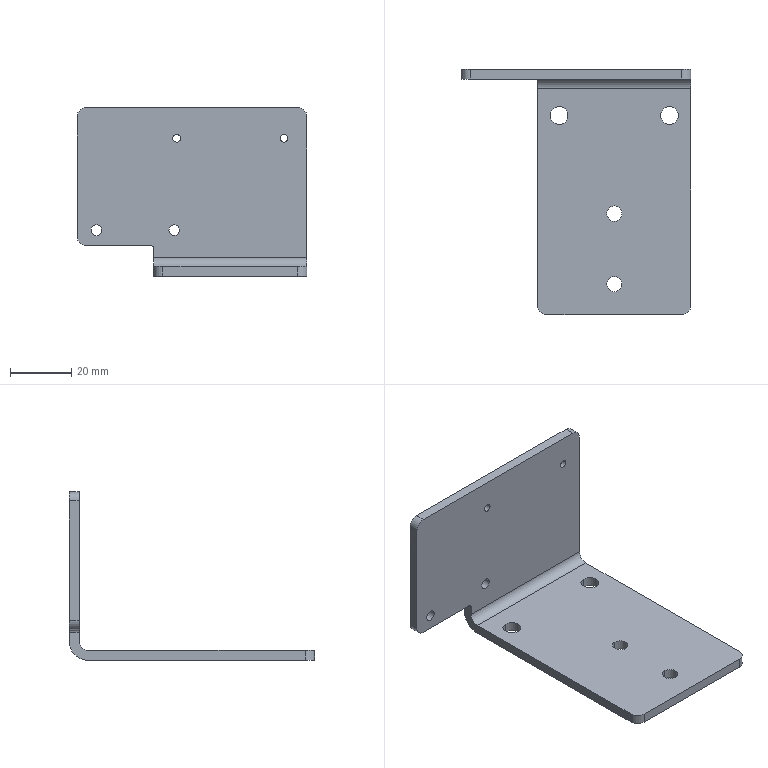Part | STEP file | J014-EBZ05-01-06-Part-1 | 1 solid | 34 faces | box 75 x 80 x 55 mm | volume 23980 mm3 | cylinder 24 | plane 10 | commonest cylinder face diameters 6 x6 2.5 x4 3.5 x4 5 x4 5.8 x4 2 x1
STEP:
#1=CARTESIAN_POINT('',(8.45,0.,15.));
#2=VERTEX_POINT('',#1);
#3=CARTESIAN_POINT('',(4.95,0.,15.));
#4=VERTEX_POINT('',#3);
#5=CARTESIAN_POINT('',(6.7,0.,15.));
#6=DIRECTION('',(0.,-1.,0.));
#7=DIRECTION('',(-1.,0.,0.));
#8=AXIS2_PLACEMENT_3D('',#5,#6,#7);
#9=CIRCLE('',#8,1.75);
#10=EDGE_CURVE('',#2,#4,#9,.T.);
#11=ORIENTED_EDGE('',*,*,#10,.F.);
#12=CARTESIAN_POINT('',(8.45,-3.2,15.));
#13=VERTEX_POINT('',#12);
#14=CARTESIAN_POINT('',(8.45,0.,15.));
#15=DIRECTION('',(0.,-1.,0.));
#16=VECTOR('',#15,1000.);
#17=LINE('',#14,#16);
#18=EDGE_CURVE('',#2,#13,#17,.T.);
#19=ORIENTED_EDGE('',*,*,#18,.T.);
#20=CARTESIAN_POINT('',(4.95,-3.2,15.));
#21=VERTEX_POINT('',#20);
#22=CARTESIAN_POINT('',(6.7,-3.2,15.));
#23=DIRECTION('',(0.,1.,0.));
#24=DIRECTION('',(1.,0.,0.));
#25=AXIS2_PLACEMENT_3D('',#22,#23,#24);
#26=CIRCLE('',#25,1.75);
#27=EDGE_CURVE('',#21,#13,#26,.T.);
#28=ORIENTED_EDGE('',*,*,#27,.F.);
#29=CARTESIAN_POINT('',(4.95,0.,15.));
#30=DIRECTION('',(0.,-1.,0.));
#31=VECTOR('',#30,1000.);
#32=LINE('',#29,#31);
#33=EDGE_CURVE('',#4,#21,#32,.T.);
#34=ORIENTED_EDGE('',*,*,#33,.F.);
#35=EDGE_LOOP('',(#11,#19,#28,#34));
#36=FACE_OUTER_BOUND('',#35,.T.);
#37=CARTESIAN_POINT('',(6.7,0.,15.));
#38=DIRECTION('',(0.,-1.,0.));
#39=DIRECTION('',(-1.,0.,0.));
#40=AXIS2_PLACEMENT_3D('',#37,#38,#39);
#41=CYLINDRICAL_SURFACE('',#40,1.75);
#42=ADVANCED_FACE('',(#36),#41,.F.);
#43=CARTESIAN_POINT('',(-16.95,0.,15.));
#44=VERTEX_POINT('',#43);
#45=CARTESIAN_POINT('',(-20.45,0.,15.));
#46=VERTEX_POINT('',#45);
#47=CARTESIAN_POINT('',(-18.7,0.,15.));
#48=DIRECTION('',(0.,-1.,0.));
#49=DIRECTION('',(-1.,0.,0.));
#50=AXIS2_PLACEMENT_3D('',#47,#48,#49);
#51=CIRCLE('',#50,1.75);
#52=EDGE_CURVE('',#44,#46,#51,.T.);
#53=ORIENTED_EDGE('',*,*,#52,.F.);
#54=CARTESIAN_POINT('',(-16.95,-3.2,15.));
#55=VERTEX_POINT('',#54);
#56=CARTESIAN_POINT('',(-16.95,0.,15.));
#57=DIRECTION('',(0.,-1.,0.));
#58=VECTOR('',#57,1000.);
#59=LINE('',#56,#58);
#60=EDGE_CURVE('',#44,#55,#59,.T.);
#61=ORIENTED_EDGE('',*,*,#60,.T.);
#62=CARTESIAN_POINT('',(-20.45,-3.2,15.));
#63=VERTEX_POINT('',#62);
#64=CARTESIAN_POINT('',(-18.7,-3.2,15.));
#65=DIRECTION('',(0.,1.,0.));
#66=DIRECTION('',(1.,0.,0.));
#67=AXIS2_PLACEMENT_3D('',#64,#65,#66);
#68=CIRCLE('',#67,1.75);
#69=EDGE_CURVE('',#63,#55,#68,.T.);
#70=ORIENTED_EDGE('',*,*,#69,.F.);
#71=CARTESIAN_POINT('',(-20.45,0.,15.));
#72=DIRECTION('',(0.,-1.,0.));
#73=VECTOR('',#72,1000.);
#74=LINE('',#71,#73);
#75=EDGE_CURVE('',#46,#63,#74,.T.);
#76=ORIENTED_EDGE('',*,*,#75,.F.);
#77=EDGE_LOOP('',(#53,#61,#70,#76));
#78=FACE_OUTER_BOUND('',#77,.T.);
#79=CARTESIAN_POINT('',(-18.7,0.,15.));
#80=DIRECTION('',(0.,-1.,0.));
#81=DIRECTION('',(-1.,0.,0.));
#82=AXIS2_PLACEMENT_3D('',#79,#80,#81);
#83=CYLINDRICAL_SURFACE('',#82,1.75);
#84=ADVANCED_FACE('',(#78),#83,.F.);
#85=CARTESIAN_POINT('',(43.75,0.,45.));
#86=VERTEX_POINT('',#85);
#87=CARTESIAN_POINT('',(41.25,0.,45.));
#88=VERTEX_POINT('',#87);
#89=CARTESIAN_POINT('',(42.5,0.,45.));
#90=DIRECTION('',(0.,-1.,0.));
#91=DIRECTION('',(-1.,0.,0.));
#92=AXIS2_PLACEMENT_3D('',#89,#90,#91);
#93=CIRCLE('',#92,1.25);
#94=EDGE_CURVE('',#86,#88,#93,.T.);
#95=ORIENTED_EDGE('',*,*,#94,.F.);
#96=CARTESIAN_POINT('',(43.75,-3.2,45.));
#97=VERTEX_POINT('',#96);
#98=CARTESIAN_POINT('',(43.75,0.,45.));
#99=DIRECTION('',(0.,-1.,0.));
#100=VECTOR('',#99,1000.);
#101=LINE('',#98,#100);
#102=EDGE_CURVE('',#86,#97,#101,.T.);
#103=ORIENTED_EDGE('',*,*,#102,.T.);
#104=CARTESIAN_POINT('',(41.25,-3.2,45.));
#105=VERTEX_POINT('',#104);
#106=CARTESIAN_POINT('',(42.5,-3.2,45.));
#107=DIRECTION('',(0.,1.,0.));
#108=DIRECTION('',(1.,0.,0.));
#109=AXIS2_PLACEMENT_3D('',#106,#107,#108);
#110=CIRCLE('',#109,1.25);
#111=EDGE_CURVE('',#105,#97,#110,.T.);
#112=ORIENTED_EDGE('',*,*,#111,.F.);
#113=CARTESIAN_POINT('',(41.25,0.,45.));
#114=DIRECTION('',(0.,-1.,0.));
#115=VECTOR('',#114,1000.);
#116=LINE('',#113,#115);
#117=EDGE_CURVE('',#88,#105,#116,.T.);
#118=ORIENTED_EDGE('',*,*,#117,.F.);
#119=EDGE_LOOP('',(#95,#103,#112,#118));
#120=FACE_OUTER_BOUND('',#119,.T.);
#121=CARTESIAN_POINT('',(42.5,0.,45.));
#122=DIRECTION('',(0.,-1.,0.));
#123=DIRECTION('',(-1.,0.,0.));
#124=AXIS2_PLACEMENT_3D('',#121,#122,#123);
#125=CYLINDRICAL_SURFACE('',#124,1.25);
#126=ADVANCED_FACE('',(#120),#125,.F.);
#127=CARTESIAN_POINT('',(8.75,0.,45.));
#128=VERTEX_POINT('',#127);
#129=CARTESIAN_POINT('',(6.25,0.,45.));
#130=VERTEX_POINT('',#129);
#131=CARTESIAN_POINT('',(7.5,0.,45.));
#132=DIRECTION('',(0.,-1.,0.));
#133=DIRECTION('',(-1.,0.,0.));
#134=AXIS2_PLACEMENT_3D('',#131,#132,#133);
#135=CIRCLE('',#134,1.25);
#136=EDGE_CURVE('',#128,#130,#135,.T.);
#137=ORIENTED_EDGE('',*,*,#136,.F.);
#138=CARTESIAN_POINT('',(8.75,-3.2,45.));
#139=VERTEX_POINT('',#138);
#140=CARTESIAN_POINT('',(8.75,0.,45.));
#141=DIRECTION('',(0.,-1.,0.));
#142=VECTOR('',#141,1000.);
#143=LINE('',#140,#142);
#144=EDGE_CURVE('',#128,#139,#143,.T.);
#145=ORIENTED_EDGE('',*,*,#144,.T.);
#146=CARTESIAN_POINT('',(6.25,-3.2,45.));
#147=VERTEX_POINT('',#146);
#148=CARTESIAN_POINT('',(7.5,-3.2,45.));
#149=DIRECTION('',(0.,1.,0.));
#150=DIRECTION('',(1.,0.,0.));
#151=AXIS2_PLACEMENT_3D('',#148,#149,#150);
#152=CIRCLE('',#151,1.25);
#153=EDGE_CURVE('',#147,#139,#152,.T.);
#154=ORIENTED_EDGE('',*,*,#153,.F.);
#155=CARTESIAN_POINT('',(6.25,0.,45.));
#156=DIRECTION('',(0.,-1.,0.));
#157=VECTOR('',#156,1000.);
#158=LINE('',#155,#157);
#159=EDGE_CURVE('',#130,#147,#158,.T.);
#160=ORIENTED_EDGE('',*,*,#159,.F.);
#161=EDGE_LOOP('',(#137,#145,#154,#160));
#162=FACE_OUTER_BOUND('',#161,.T.);
#163=CARTESIAN_POINT('',(7.5,0.,45.));
#164=DIRECTION('',(0.,-1.,0.));
#165=DIRECTION('',(-1.,0.,0.));
#166=AXIS2_PLACEMENT_3D('',#163,#164,#165);
#167=CYLINDRICAL_SURFACE('',#166,1.25);
#168=ADVANCED_FACE('',(#162),#167,.F.);
#169=CARTESIAN_POINT('',(25.,-67.5,3.2));
#170=VERTEX_POINT('',#169);
#171=CARTESIAN_POINT('',(25.,-72.5,3.2));
#172=VERTEX_POINT('',#171);
#173=CARTESIAN_POINT('',(25.,-70.,3.2));
#174=DIRECTION('',(0.,0.,-1.));
#175=DIRECTION('',(0.,-1.,0.));
#176=AXIS2_PLACEMENT_3D('',#173,#174,#175);
#177=CIRCLE('',#176,2.5);
#178=EDGE_CURVE('',#170,#172,#177,.T.);
#179=ORIENTED_EDGE('',*,*,#178,.F.);
#180=CARTESIAN_POINT('',(25.,-67.5,0.));
#181=VERTEX_POINT('',#180);
#182=CARTESIAN_POINT('',(25.,-67.5,3.2));
#183=DIRECTION('',(0.,0.,-1.));
#184=VECTOR('',#183,1000.);
#185=LINE('',#182,#184);
#186=EDGE_CURVE('',#170,#181,#185,.T.);
#187=ORIENTED_EDGE('',*,*,#186,.T.);
#188=CARTESIAN_POINT('',(25.,-72.5,0.));
#189=VERTEX_POINT('',#188);
#190=CARTESIAN_POINT('',(25.,-70.,0.));
#191=DIRECTION('',(0.,0.,1.));
#192=DIRECTION('',(0.,1.,0.));
#193=AXIS2_PLACEMENT_3D('',#190,#191,#192);
#194=CIRCLE('',#193,2.5);
#195=EDGE_CURVE('',#189,#181,#194,.T.);
#196=ORIENTED_EDGE('',*,*,#195,.F.);
#197=CARTESIAN_POINT('',(25.,-72.5,3.2));
#198=DIRECTION('',(0.,0.,-1.));
#199=VECTOR('',#198,1000.);
#200=LINE('',#197,#199);
#201=EDGE_CURVE('',#172,#189,#200,.T.);
#202=ORIENTED_EDGE('',*,*,#201,.F.);
#203=EDGE_LOOP('',(#179,#187,#196,#202));
#204=FACE_OUTER_BOUND('',#203,.T.);
#205=CARTESIAN_POINT('',(25.,-70.,3.2));
#206=DIRECTION('',(0.,0.,-1.));
#207=DIRECTION('',(0.,-1.,0.));
#208=AXIS2_PLACEMENT_3D('',#205,#206,#207);
#209=CYLINDRICAL_SURFACE('',#208,2.5);
#210=ADVANCED_FACE('',(#204),#209,.F.);
#211=CARTESIAN_POINT('',(25.,-44.5,3.2));
#212=VERTEX_POINT('',#211);
#213=CARTESIAN_POINT('',(25.,-49.5,3.2));
#214=VERTEX_POINT('',#213);
#215=CARTESIAN_POINT('',(25.,-47.,3.2));
#216=DIRECTION('',(0.,0.,-1.));
#217=DIRECTION('',(0.,-1.,0.));
#218=AXIS2_PLACEMENT_3D('',#215,#216,#217);
#219=CIRCLE('',#218,2.5);
#220=EDGE_CURVE('',#212,#214,#219,.T.);
#221=ORIENTED_EDGE('',*,*,#220,.F.);
#222=CARTESIAN_POINT('',(25.,-44.5,0.));
#223=VERTEX_POINT('',#222);
#224=CARTESIAN_POINT('',(25.,-44.5,3.2));
#225=DIRECTION('',(0.,0.,-1.));
#226=VECTOR('',#225,1000.);
#227=LINE('',#224,#226);
#228=EDGE_CURVE('',#212,#223,#227,.T.);
#229=ORIENTED_EDGE('',*,*,#228,.T.);
#230=CARTESIAN_POINT('',(25.,-49.5,0.));
#231=VERTEX_POINT('',#230);
#232=CARTESIAN_POINT('',(25.,-47.,0.));
#233=DIRECTION('',(0.,0.,1.));
#234=DIRECTION('',(0.,1.,0.));
#235=AXIS2_PLACEMENT_3D('',#232,#233,#234);
#236=CIRCLE('',#235,2.5);
#237=EDGE_CURVE('',#231,#223,#236,.T.);
#238=ORIENTED_EDGE('',*,*,#237,.F.);
#239=CARTESIAN_POINT('',(25.,-49.5,3.2));
#240=DIRECTION('',(0.,0.,-1.));
#241=VECTOR('',#240,1000.);
#242=LINE('',#239,#241);
#243=EDGE_CURVE('',#214,#231,#242,.T.);
#244=ORIENTED_EDGE('',*,*,#243,.F.);
#245=EDGE_LOOP('',(#221,#229,#238,#244));
#246=FACE_OUTER_BOUND('',#245,.T.);
#247=CARTESIAN_POINT('',(25.,-47.,3.2));
#248=DIRECTION('',(0.,0.,-1.));
#249=DIRECTION('',(0.,-1.,0.));
#250=AXIS2_PLACEMENT_3D('',#247,#248,#249);
#251=CYLINDRICAL_SURFACE('',#250,2.5);
#252=ADVANCED_FACE('',(#246),#251,.F.);
#253=CARTESIAN_POINT('',(43.,-12.1,3.2));
#254=VERTEX_POINT('',#253);
#255=CARTESIAN_POINT('',(43.,-17.9,3.2));
#256=VERTEX_POINT('',#255);
#257=CARTESIAN_POINT('',(43.,-15.,3.2));
#258=DIRECTION('',(0.,0.,-1.));
#259=DIRECTION('',(0.,-1.,0.));
#260=AXIS2_PLACEMENT_3D('',#257,#258,#259);
#261=CIRCLE('',#260,2.9);
#262=EDGE_CURVE('',#254,#256,#261,.T.);
#263=ORIENTED_EDGE('',*,*,#262,.F.);
#264=CARTESIAN_POINT('',(43.,-12.1,0.));
#265=VERTEX_POINT('',#264);
#266=CARTESIAN_POINT('',(43.,-12.1,3.2));
#267=DIRECTION('',(0.,0.,-1.));
#268=VECTOR('',#267,1000.);
#269=LINE('',#266,#268);
#270=EDGE_CURVE('',#254,#265,#269,.T.);
#271=ORIENTED_EDGE('',*,*,#270,.T.);
#272=CARTESIAN_POINT('',(43.,-17.9,0.));
#273=VERTEX_POINT('',#272);
#274=CARTESIAN_POINT('',(43.,-15.,0.));
#275=DIRECTION('',(0.,0.,-1.));
#276=DIRECTION('',(0.,-1.,0.));
#277=AXIS2_PLACEMENT_3D('',#274,#275,#276);
#278=CIRCLE('',#277,2.9);
#279=EDGE_CURVE('',#265,#273,#278,.T.);
#280=ORIENTED_EDGE('',*,*,#279,.T.);
#281=CARTESIAN_POINT('',(43.,-17.9,3.2));
#282=DIRECTION('',(0.,0.,-1.));
#283=VECTOR('',#282,1000.);
#284=LINE('',#281,#283);
#285=EDGE_CURVE('',#256,#273,#284,.T.);
#286=ORIENTED_EDGE('',*,*,#285,.F.);
#287=EDGE_LOOP('',(#263,#271,#280,#286));
#288=FACE_OUTER_BOUND('',#287,.T.);
#289=CARTESIAN_POINT('',(43.,-15.,3.2));
#290=DIRECTION('',(0.,0.,-1.));
#291=DIRECTION('',(0.,-1.,0.));
#292=AXIS2_PLACEMENT_3D('',#289,#290,#291);
#293=CYLINDRICAL_SURFACE('',#292,2.9);
#294=ADVANCED_FACE('',(#288),#293,.F.);
#295=CARTESIAN_POINT('',(7.,-12.1,3.2));
#296=VERTEX_POINT('',#295);
#297=CARTESIAN_POINT('',(7.,-17.9,3.2));
#298=VERTEX_POINT('',#297);
#299=CARTESIAN_POINT('',(7.,-15.,3.2));
#300=DIRECTION('',(0.,0.,-1.));
#301=DIRECTION('',(0.,-1.,0.));
#302=AXIS2_PLACEMENT_3D('',#299,#300,#301);
#303=CIRCLE('',#302,2.9);
#304=EDGE_CURVE('',#296,#298,#303,.T.);
#305=ORIENTED_EDGE('',*,*,#304,.F.);
#306=CARTESIAN_POINT('',(7.,-12.1,0.));
#307=VERTEX_POINT('',#306);
#308=CARTESIAN_POINT('',(7.,-12.1,3.2));
#309=DIRECTION('',(0.,0.,-1.));
#310=VECTOR('',#309,1000.);
#311=LINE('',#308,#310);
#312=EDGE_CURVE('',#296,#307,#311,.T.);
#313=ORIENTED_EDGE('',*,*,#312,.T.);
#314=CARTESIAN_POINT('',(7.,-17.9,0.));
#315=VERTEX_POINT('',#314);
#316=CARTESIAN_POINT('',(7.,-15.,0.));
#317=DIRECTION('',(0.,0.,-1.));
#318=DIRECTION('',(0.,-1.,0.));
#319=AXIS2_PLACEMENT_3D('',#316,#317,#318);
#320=CIRCLE('',#319,2.9);
#321=EDGE_CURVE('',#307,#315,#320,.T.);
#322=ORIENTED_EDGE('',*,*,#321,.T.);
#323=CARTESIAN_POINT('',(7.,-17.9,3.2));
#324=DIRECTION('',(0.,0.,-1.));
#325=VECTOR('',#324,1000.);
#326=LINE('',#323,#325);
#327=EDGE_CURVE('',#298,#315,#326,.T.);
#328=ORIENTED_EDGE('',*,*,#327,.F.);
#329=EDGE_LOOP('',(#305,#313,#322,#328));
#330=FACE_OUTER_BOUND('',#329,.T.);
#331=CARTESIAN_POINT('',(7.,-15.,3.2));
#332=DIRECTION('',(0.,0.,-1.));
#333=DIRECTION('',(0.,-1.,0.));
#334=AXIS2_PLACEMENT_3D('',#331,#332,#333);
#335=CYLINDRICAL_SURFACE('',#334,2.9);
#336=ADVANCED_FACE('',(#330),#335,.F.);
#337=CARTESIAN_POINT('',(0.,-3.2,6.2));
#338=VERTEX_POINT('',#337);
#339=CARTESIAN_POINT('',(0.,-3.2,9.));
#340=VERTEX_POINT('',#339);
#341=CARTESIAN_POINT('',(0.,-3.2,3.2));
#342=DIRECTION('',(0.,0.,1.));
#343=VECTOR('',#342,1000.);
#344=LINE('',#341,#343);
#345=EDGE_CURVE('',#338,#340,#344,.T.);
#346=ORIENTED_EDGE('',*,*,#345,.T.);
#347=CARTESIAN_POINT('',(0.,0.,9.));
#348=VERTEX_POINT('',#347);
#349=CARTESIAN_POINT('',(0.,0.,9.));
#350=DIRECTION('',(0.,1.,0.));
#351=VECTOR('',#350,1000.);
#352=LINE('',#349,#351);
#353=EDGE_CURVE('',#340,#348,#352,.T.);
#354=ORIENTED_EDGE('',*,*,#353,.T.);
#355=CARTESIAN_POINT('',(0.,0.,6.));
#356=VERTEX_POINT('',#355);
#357=CARTESIAN_POINT('',(0.,0.,0.));
#358=DIRECTION('',(0.,0.,1.));
#359=VECTOR('',#358,1000.);
#360=LINE('',#357,#359);
#361=EDGE_CURVE('',#356,#348,#360,.T.);
#362=ORIENTED_EDGE('',*,*,#361,.F.);
#363=CARTESIAN_POINT('',(0.,-6.,0.));
#364=VERTEX_POINT('',#363);
#365=CARTESIAN_POINT('',(0.,-6.,6.));
#366=DIRECTION('',(-1.,0.,0.));
#367=DIRECTION('',(0.,1.,0.));
#368=AXIS2_PLACEMENT_3D('',#365,#366,#367);
#369=CIRCLE('',#368,6.);
#370=EDGE_CURVE('',#356,#364,#369,.T.);
#371=ORIENTED_EDGE('',*,*,#370,.T.);
#372=CARTESIAN_POINT('',(0.,-77.,0.));
#373=VERTEX_POINT('',#372);
#374=CARTESIAN_POINT('',(0.,-40.,0.));
#375=DIRECTION('',(0.,-1.,0.));
#376=VECTOR('',#375,1000.);
#377=LINE('',#374,#376);
#378=EDGE_CURVE('',#364,#373,#377,.T.);
#379=ORIENTED_EDGE('',*,*,#378,.T.);
#380=CARTESIAN_POINT('',(0.,-77.,3.2));
#381=VERTEX_POINT('',#380);
#382=CARTESIAN_POINT('',(0.,-77.,0.));
#383=DIRECTION('',(0.,0.,1.));
#384=VECTOR('',#383,1000.);
#385=LINE('',#382,#384);
#386=EDGE_CURVE('',#373,#381,#385,.T.);
#387=ORIENTED_EDGE('',*,*,#386,.T.);
#388=CARTESIAN_POINT('',(0.,-6.2,3.2));
#389=VERTEX_POINT('',#388);
#390=CARTESIAN_POINT('',(0.,-40.,3.2));
#391=DIRECTION('',(0.,1.,0.));
#392=VECTOR('',#391,1000.);
#393=LINE('',#390,#392);
#394=EDGE_CURVE('',#381,#389,#393,.T.);
#395=ORIENTED_EDGE('',*,*,#394,.T.);
#396=CARTESIAN_POINT('',(0.,-6.2,6.2));
#397=DIRECTION('',(1.,0.,0.));
#398=DIRECTION('',(0.,1.,0.));
#399=AXIS2_PLACEMENT_3D('',#396,#397,#398);
#400=CIRCLE('',#399,3.);
#401=EDGE_CURVE('',#389,#338,#400,.T.);
#402=ORIENTED_EDGE('',*,*,#401,.T.);
#403=EDGE_LOOP('',(#346,#354,#362,#371,#379,#387,#395,#402));
#404=FACE_OUTER_BOUND('',#403,.T.);
#405=CARTESIAN_POINT('',(0.,-40.,0.));
#406=DIRECTION('',(-1.,0.,0.));
#407=DIRECTION('',(0.,0.,1.));
#408=AXIS2_PLACEMENT_3D('',#405,#406,#407);
#409=PLANE('',#408);
#410=ADVANCED_FACE('',(#404),#409,.T.);
#411=CARTESIAN_POINT('',(25.,-70.,3.2));
#412=DIRECTION('',(0.,0.,-1.));
#413=DIRECTION('',(0.,-1.,0.));
#414=AXIS2_PLACEMENT_3D('',#411,#412,#413);
#415=CIRCLE('',#414,2.5);
#416=EDGE_CURVE('',#172,#170,#415,.T.);
#417=ORIENTED_EDGE('',*,*,#416,.T.);
#418=ORIENTED_EDGE('',*,*,#178,.T.);
#419=EDGE_LOOP('',(#417,#418));
#420=FACE_BOUND('',#419,.T.);
#421=CARTESIAN_POINT('',(25.,-47.,3.2));
#422=DIRECTION('',(0.,0.,-1.));
#423=DIRECTION('',(0.,-1.,0.));
#424=AXIS2_PLACEMENT_3D('',#421,#422,#423);
#425=CIRCLE('',#424,2.5);
#426=EDGE_CURVE('',#214,#212,#425,.T.);
#427=ORIENTED_EDGE('',*,*,#426,.T.);
#428=ORIENTED_EDGE('',*,*,#220,.T.);
#429=EDGE_LOOP('',(#427,#428));
#430=FACE_BOUND('',#429,.T.);
#431=CARTESIAN_POINT('',(43.,-15.,3.2));
#432=DIRECTION('',(0.,0.,-1.));
#433=DIRECTION('',(0.,-1.,0.));
#434=AXIS2_PLACEMENT_3D('',#431,#432,#433);
#435=CIRCLE('',#434,2.9);
#436=EDGE_CURVE('',#256,#254,#435,.T.);
#437=ORIENTED_EDGE('',*,*,#436,.T.);
#438=ORIENTED_EDGE('',*,*,#262,.T.);
#439=EDGE_LOOP('',(#437,#438));
#440=FACE_BOUND('',#439,.T.);
#441=CARTESIAN_POINT('',(7.,-15.,3.2));
#442=DIRECTION('',(0.,0.,-1.));
#443=DIRECTION('',(0.,-1.,0.));
#444=AXIS2_PLACEMENT_3D('',#441,#442,#443);
#445=CIRCLE('',#444,2.9);
#446=EDGE_CURVE('',#298,#296,#445,.T.);
#447=ORIENTED_EDGE('',*,*,#446,.T.);
#448=ORIENTED_EDGE('',*,*,#304,.T.);
#449=EDGE_LOOP('',(#447,#448));
#450=FACE_BOUND('',#449,.T.);
#451=ORIENTED_EDGE('',*,*,#394,.F.);
#452=CARTESIAN_POINT('',(3.,-80.,3.2));
#453=VERTEX_POINT('',#452);
#454=CARTESIAN_POINT('',(3.,-77.,3.2));
#455=DIRECTION('',(0.,0.,1.));
#456=DIRECTION('',(0.,1.,0.));
#457=AXIS2_PLACEMENT_3D('',#454,#455,#456);
#458=CIRCLE('',#457,3.);
#459=EDGE_CURVE('',#381,#453,#458,.T.);
#460=ORIENTED_EDGE('',*,*,#459,.T.);
#461=CARTESIAN_POINT('',(47.,-80.,3.2));
#462=VERTEX_POINT('',#461);
#463=CARTESIAN_POINT('',(25.,-80.,3.2));
#464=DIRECTION('',(-1.,0.,0.));
#465=VECTOR('',#464,1000.);
#466=LINE('',#463,#465);
#467=EDGE_CURVE('',#462,#453,#466,.T.);
#468=ORIENTED_EDGE('',*,*,#467,.F.);
#469=CARTESIAN_POINT('',(50.,-77.,3.2));
#470=VERTEX_POINT('',#469);
#471=CARTESIAN_POINT('',(47.,-77.,3.2));
#472=DIRECTION('',(0.,0.,1.));
#473=DIRECTION('',(0.,1.,0.));
#474=AXIS2_PLACEMENT_3D('',#471,#472,#473);
#475=CIRCLE('',#474,3.);
#476=EDGE_CURVE('',#462,#470,#475,.T.);
#477=ORIENTED_EDGE('',*,*,#476,.T.);
#478=CARTESIAN_POINT('',(50.,-6.2,3.2));
#479=VERTEX_POINT('',#478);
#480=CARTESIAN_POINT('',(50.,-40.,3.2));
#481=DIRECTION('',(0.,-1.,0.));
#482=VECTOR('',#481,1000.);
#483=LINE('',#480,#482);
#484=EDGE_CURVE('',#479,#470,#483,.T.);
#485=ORIENTED_EDGE('',*,*,#484,.F.);
#486=CARTESIAN_POINT('',(0.,-6.2,3.2));
#487=DIRECTION('',(-1.,0.,0.));
#488=VECTOR('',#487,1000.);
#489=LINE('',#486,#488);
#490=EDGE_CURVE('',#479,#389,#489,.T.);
#491=ORIENTED_EDGE('',*,*,#490,.T.);
#492=EDGE_LOOP('',(#451,#460,#468,#477,#485,#491));
#493=FACE_OUTER_BOUND('',#492,.T.);
#494=CARTESIAN_POINT('',(25.,-40.,3.2));
#495=DIRECTION('',(0.,0.,1.));
#496=DIRECTION('',(0.,1.,0.));
#497=AXIS2_PLACEMENT_3D('',#494,#495,#496);
#498=PLANE('',#497);
#499=ADVANCED_FACE('',(#420,#430,#440,#450,#493),#498,.T.);
#500=CARTESIAN_POINT('',(50.,0.,6.));
#501=VERTEX_POINT('',#500);
#502=CARTESIAN_POINT('',(50.,0.,52.));
#503=VERTEX_POINT('',#502);
#504=CARTESIAN_POINT('',(50.,0.,0.));
#505=DIRECTION('',(0.,0.,1.));
#506=VECTOR('',#505,1000.);
#507=LINE('',#504,#506);
#508=EDGE_CURVE('',#501,#503,#507,.T.);
#509=ORIENTED_EDGE('',*,*,#508,.T.);
#510=CARTESIAN_POINT('',(50.,-3.2,52.));
#511=VERTEX_POINT('',#510);
#512=CARTESIAN_POINT('',(50.,-40.,52.));
#513=DIRECTION('',(0.,-1.,0.));
#514=VECTOR('',#513,1000.);
#515=LINE('',#512,#514);
#516=EDGE_CURVE('',#503,#511,#515,.T.);
#517=ORIENTED_EDGE('',*,*,#516,.T.);
#518=CARTESIAN_POINT('',(50.,-3.2,6.2));
#519=VERTEX_POINT('',#518);
#520=CARTESIAN_POINT('',(50.,-3.2,3.2));
#521=DIRECTION('',(0.,0.,1.));
#522=VECTOR('',#521,1000.);
#523=LINE('',#520,#522);
#524=EDGE_CURVE('',#519,#511,#523,.T.);
#525=ORIENTED_EDGE('',*,*,#524,.F.);
#526=CARTESIAN_POINT('',(50.,-6.2,6.2));
#527=DIRECTION('',(-1.,0.,0.));
#528=DIRECTION('',(0.,-1.,0.));
#529=AXIS2_PLACEMENT_3D('',#526,#527,#528);
#530=CIRCLE('',#529,3.);
#531=EDGE_CURVE('',#519,#479,#530,.T.);
#532=ORIENTED_EDGE('',*,*,#531,.T.);
#533=ORIENTED_EDGE('',*,*,#484,.T.);
#534=CARTESIAN_POINT('',(50.,-77.,0.));
#535=VERTEX_POINT('',#534);
#536=CARTESIAN_POINT('',(50.,-77.,0.));
#537=DIRECTION('',(0.,0.,-1.));
#538=VECTOR('',#537,1000.);
#539=LINE('',#536,#538);
#540=EDGE_CURVE('',#470,#535,#539,.T.);
#541=ORIENTED_EDGE('',*,*,#540,.T.);
#542=CARTESIAN_POINT('',(50.,-6.,0.));
#543=VERTEX_POINT('',#542);
#544=CARTESIAN_POINT('',(50.,-40.,0.));
#545=DIRECTION('',(0.,1.,0.));
#546=VECTOR('',#545,1000.);
#547=LINE('',#544,#546);
#548=EDGE_CURVE('',#535,#543,#547,.T.);
#549=ORIENTED_EDGE('',*,*,#548,.T.);
#550=CARTESIAN_POINT('',(50.,-6.,6.));
#551=DIRECTION('',(1.,0.,0.));
#552=DIRECTION('',(0.,-1.,0.));
#553=AXIS2_PLACEMENT_3D('',#550,#551,#552);
#554=CIRCLE('',#553,6.);
#555=EDGE_CURVE('',#543,#501,#554,.T.);
#556=ORIENTED_EDGE('',*,*,#555,.T.);
#557=EDGE_LOOP('',(#509,#517,#525,#532,#533,#541,#549,#556));
#558=FACE_OUTER_BOUND('',#557,.T.);
#559=CARTESIAN_POINT('',(50.,-40.,0.));
#560=DIRECTION('',(1.,0.,0.));
#561=DIRECTION('',(0.,0.,-1.));
#562=AXIS2_PLACEMENT_3D('',#559,#560,#561);
#563=PLANE('',#562);
#564=ADVANCED_FACE('',(#558),#563,.T.);
#565=ORIENTED_EDGE('',*,*,#467,.T.);
#566=CARTESIAN_POINT('',(3.,-80.,0.));
#567=VERTEX_POINT('',#566);
#568=CARTESIAN_POINT('',(3.,-80.,0.));
#569=DIRECTION('',(0.,0.,-1.));
#570=VECTOR('',#569,1000.);
#571=LINE('',#568,#570);
#572=EDGE_CURVE('',#453,#567,#571,.T.);
#573=ORIENTED_EDGE('',*,*,#572,.T.);
#574=CARTESIAN_POINT('',(47.,-80.,0.));
#575=VERTEX_POINT('',#574);
#576=CARTESIAN_POINT('',(25.,-80.,0.));
#577=DIRECTION('',(1.,0.,0.));
#578=VECTOR('',#577,1000.);
#579=LINE('',#576,#578);
#580=EDGE_CURVE('',#567,#575,#579,.T.);
#581=ORIENTED_EDGE('',*,*,#580,.T.);
#582=CARTESIAN_POINT('',(47.,-80.,0.));
#583=DIRECTION('',(0.,0.,1.));
#584=VECTOR('',#583,1000.);
#585=LINE('',#582,#584);
#586=EDGE_CURVE('',#575,#462,#585,.T.);
#587=ORIENTED_EDGE('',*,*,#586,.T.);
#588=EDGE_LOOP('',(#565,#573,#581,#587));
#589=FACE_OUTER_BOUND('',#588,.T.);
#590=CARTESIAN_POINT('',(25.,-80.,0.));
#591=DIRECTION('',(0.,-1.,0.));
#592=DIRECTION('',(0.,0.,1.));
#593=AXIS2_PLACEMENT_3D('',#590,#591,#592);
#594=PLANE('',#593);
#595=ADVANCED_FACE('',(#589),#594,.T.);
#596=ORIENTED_EDGE('',*,*,#195,.T.);
#597=CARTESIAN_POINT('',(25.,-70.,0.));
#598=DIRECTION('',(0.,0.,1.));
#599=DIRECTION('',(0.,1.,0.));
#600=AXIS2_PLACEMENT_3D('',#597,#598,#599);
#601=CIRCLE('',#600,2.5);
#602=EDGE_CURVE('',#181,#189,#601,.T.);
#603=ORIENTED_EDGE('',*,*,#602,.T.);
#604=EDGE_LOOP('',(#596,#603));
#605=FACE_BOUND('',#604,.T.);
#606=ORIENTED_EDGE('',*,*,#237,.T.);
#607=CARTESIAN_POINT('',(25.,-47.,0.));
#608=DIRECTION('',(0.,0.,1.));
#609=DIRECTION('',(0.,1.,0.));
#610=AXIS2_PLACEMENT_3D('',#607,#608,#609);
#611=CIRCLE('',#610,2.5);
#612=EDGE_CURVE('',#223,#231,#611,.T.);
#613=ORIENTED_EDGE('',*,*,#612,.T.);
#614=EDGE_LOOP('',(#606,#613));
#615=FACE_BOUND('',#614,.T.);
#616=CARTESIAN_POINT('',(43.,-15.,0.));
#617=DIRECTION('',(0.,0.,-1.));
#618=DIRECTION('',(0.,-1.,0.));
#619=AXIS2_PLACEMENT_3D('',#616,#617,#618);
#620=CIRCLE('',#619,2.9);
#621=EDGE_CURVE('',#273,#265,#620,.T.);
#622=ORIENTED_EDGE('',*,*,#621,.F.);
#623=ORIENTED_EDGE('',*,*,#279,.F.);
#624=EDGE_LOOP('',(#622,#623));
#625=FACE_BOUND('',#624,.T.);
#626=CARTESIAN_POINT('',(7.,-15.,0.));
#627=DIRECTION('',(0.,0.,-1.));
#628=DIRECTION('',(0.,-1.,0.));
#629=AXIS2_PLACEMENT_3D('',#626,#627,#628);
#630=CIRCLE('',#629,2.9);
#631=EDGE_CURVE('',#315,#307,#630,.T.);
#632=ORIENTED_EDGE('',*,*,#631,.F.);
#633=ORIENTED_EDGE('',*,*,#321,.F.);
#634=EDGE_LOOP('',(#632,#633));
#635=FACE_BOUND('',#634,.T.);
#636=ORIENTED_EDGE('',*,*,#580,.F.);
#637=CARTESIAN_POINT('',(3.,-77.,0.));
#638=DIRECTION('',(0.,0.,-1.));
#639=DIRECTION('',(0.,-1.,0.));
#640=AXIS2_PLACEMENT_3D('',#637,#638,#639);
#641=CIRCLE('',#640,3.);
#642=EDGE_CURVE('',#567,#373,#641,.T.);
#643=ORIENTED_EDGE('',*,*,#642,.T.);
#644=ORIENTED_EDGE('',*,*,#378,.F.);
#645=CARTESIAN_POINT('',(25.,-6.,0.));
#646=DIRECTION('',(1.,0.,0.));
#647=VECTOR('',#646,1000.);
#648=LINE('',#645,#647);
#649=EDGE_CURVE('',#364,#543,#648,.T.);
#650=ORIENTED_EDGE('',*,*,#649,.T.);
#651=ORIENTED_EDGE('',*,*,#548,.F.);
#652=CARTESIAN_POINT('',(47.,-77.,0.));
#653=DIRECTION('',(0.,0.,-1.));
#654=DIRECTION('',(0.,-1.,0.));
#655=AXIS2_PLACEMENT_3D('',#652,#653,#654);
#656=CIRCLE('',#655,3.);
#657=EDGE_CURVE('',#535,#575,#656,.T.);
#658=ORIENTED_EDGE('',*,*,#657,.T.);
#659=EDGE_LOOP('',(#636,#643,#644,#650,#651,#658));
#660=FACE_OUTER_BOUND('',#659,.T.);
#661=CARTESIAN_POINT('',(25.,-40.,0.));
#662=DIRECTION('',(0.,0.,-1.));
#663=DIRECTION('',(0.,-1.,0.));
#664=AXIS2_PLACEMENT_3D('',#661,#662,#663);
#665=PLANE('',#664);
#666=ADVANCED_FACE('',(#605,#615,#625,#635,#660),#665,.T.);
#667=CARTESIAN_POINT('',(6.7,0.,15.));
#668=DIRECTION('',(0.,-1.,0.));
#669=DIRECTION('',(-1.,0.,0.));
#670=AXIS2_PLACEMENT_3D('',#667,#668,#669);
#671=CIRCLE('',#670,1.75);
#672=EDGE_CURVE('',#4,#2,#671,.T.);
#673=ORIENTED_EDGE('',*,*,#672,.T.);
#674=ORIENTED_EDGE('',*,*,#10,.T.);
#675=EDGE_LOOP('',(#673,#674));
#676=FACE_BOUND('',#675,.T.);
#677=CARTESIAN_POINT('',(-18.7,0.,15.));
#678=DIRECTION('',(0.,-1.,0.));
#679=DIRECTION('',(-1.,0.,0.));
#680=AXIS2_PLACEMENT_3D('',#677,#678,#679);
#681=CIRCLE('',#680,1.75);
#682=EDGE_CURVE('',#46,#44,#681,.T.);
#683=ORIENTED_EDGE('',*,*,#682,.T.);
#684=ORIENTED_EDGE('',*,*,#52,.T.);
#685=EDGE_LOOP('',(#683,#684));
#686=FACE_BOUND('',#685,.T.);
#687=CARTESIAN_POINT('',(42.5,0.,45.));
#688=DIRECTION('',(0.,-1.,0.));
#689=DIRECTION('',(-1.,0.,0.));
#690=AXIS2_PLACEMENT_3D('',#687,#688,#689);
#691=CIRCLE('',#690,1.25);
#692=EDGE_CURVE('',#88,#86,#691,.T.);
#693=ORIENTED_EDGE('',*,*,#692,.T.);
#694=ORIENTED_EDGE('',*,*,#94,.T.);
#695=EDGE_LOOP('',(#693,#694));
#696=FACE_BOUND('',#695,.T.);
#697=CARTESIAN_POINT('',(7.5,0.,45.));
#698=DIRECTION('',(0.,-1.,0.));
#699=DIRECTION('',(-1.,0.,0.));
#700=AXIS2_PLACEMENT_3D('',#697,#698,#699);
#701=CIRCLE('',#700,1.25);
#702=EDGE_CURVE('',#130,#128,#701,.T.);
#703=ORIENTED_EDGE('',*,*,#702,.T.);
#704=ORIENTED_EDGE('',*,*,#136,.T.);
#705=EDGE_LOOP('',(#703,#704));
#706=FACE_BOUND('',#705,.T.);
#707=CARTESIAN_POINT('',(-22.,0.,55.));
#708=VERTEX_POINT('',#707);
#709=CARTESIAN_POINT('',(47.,0.,55.));
#710=VERTEX_POINT('',#709);
#711=CARTESIAN_POINT('',(25.,0.,55.));
#712=DIRECTION('',(1.,0.,0.));
#713=VECTOR('',#712,1000.);
#714=LINE('',#711,#713);
#715=EDGE_CURVE('',#708,#710,#714,.T.);
#716=ORIENTED_EDGE('',*,*,#715,.T.);
#717=CARTESIAN_POINT('',(47.,0.,52.));
#718=DIRECTION('',(0.,1.,0.));
#719=DIRECTION('',(1.,0.,0.));
#720=AXIS2_PLACEMENT_3D('',#717,#718,#719);
#721=CIRCLE('',#720,3.);
#722=EDGE_CURVE('',#710,#503,#721,.T.);
#723=ORIENTED_EDGE('',*,*,#722,.T.);
#724=ORIENTED_EDGE('',*,*,#508,.F.);
#725=CARTESIAN_POINT('',(25.,0.,6.));
#726=DIRECTION('',(-1.,0.,0.));
#727=VECTOR('',#726,1000.);
#728=LINE('',#725,#727);
#729=EDGE_CURVE('',#501,#356,#728,.T.);
#730=ORIENTED_EDGE('',*,*,#729,.T.);
#731=ORIENTED_EDGE('',*,*,#361,.T.);
#732=CARTESIAN_POINT('',(-1.,0.,10.));
#733=VERTEX_POINT('',#732);
#734=CARTESIAN_POINT('',(-1.,0.,9.));
#735=DIRECTION('',(0.,-1.,0.));
#736=DIRECTION('',(1.,0.,0.));
#737=AXIS2_PLACEMENT_3D('',#734,#735,#736);
#738=CIRCLE('',#737,1.);
#739=EDGE_CURVE('',#348,#733,#738,.T.);
#740=ORIENTED_EDGE('',*,*,#739,.T.);
#741=CARTESIAN_POINT('',(-22.,0.,10.));
#742=VERTEX_POINT('',#741);
#743=CARTESIAN_POINT('',(-12.5,0.,10.));
#744=DIRECTION('',(1.,0.,0.));
#745=VECTOR('',#744,1000.);
#746=LINE('',#743,#745);
#747=EDGE_CURVE('',#742,#733,#746,.T.);
#748=ORIENTED_EDGE('',*,*,#747,.F.);
#749=CARTESIAN_POINT('',(-25.,0.,13.));
#750=VERTEX_POINT('',#749);
#751=CARTESIAN_POINT('',(-22.,0.,13.));
#752=DIRECTION('',(0.,1.,0.));
#753=DIRECTION('',(1.,0.,0.));
#754=AXIS2_PLACEMENT_3D('',#751,#752,#753);
#755=CIRCLE('',#754,3.);
#756=EDGE_CURVE('',#742,#750,#755,.T.);
#757=ORIENTED_EDGE('',*,*,#756,.T.);
#758=CARTESIAN_POINT('',(-25.,0.,52.));
#759=VERTEX_POINT('',#758);
#760=CARTESIAN_POINT('',(-25.,0.,32.5));
#761=DIRECTION('',(0.,0.,-1.));
#762=VECTOR('',#761,1000.);
#763=LINE('',#760,#762);
#764=EDGE_CURVE('',#759,#750,#763,.T.);
#765=ORIENTED_EDGE('',*,*,#764,.F.);
#766=CARTESIAN_POINT('',(-22.,0.,52.));
#767=DIRECTION('',(0.,1.,0.));
#768=DIRECTION('',(1.,0.,0.));
#769=AXIS2_PLACEMENT_3D('',#766,#767,#768);
#770=CIRCLE('',#769,3.);
#771=EDGE_CURVE('',#759,#708,#770,.T.);
#772=ORIENTED_EDGE('',*,*,#771,.T.);
#773=EDGE_LOOP('',(#716,#723,#724,#730,#731,#740,#748,#757,#765,#772));
#774=FACE_OUTER_BOUND('',#773,.T.);
#775=CARTESIAN_POINT('',(25.,0.,0.));
#776=DIRECTION('',(0.,1.,0.));
#777=DIRECTION('',(0.,0.,-1.));
#778=AXIS2_PLACEMENT_3D('',#775,#776,#777);
#779=PLANE('',#778);
#780=ADVANCED_FACE('',(#676,#686,#696,#706,#774),#779,.T.);
#781=CARTESIAN_POINT('',(47.,-3.2,55.));
#782=VERTEX_POINT('',#781);
#783=CARTESIAN_POINT('',(-22.,-3.2,55.));
#784=VERTEX_POINT('',#783);
#785=CARTESIAN_POINT('',(25.,-3.2,55.));
#786=DIRECTION('',(-1.,0.,0.));
#787=VECTOR('',#786,1000.);
#788=LINE('',#785,#787);
#789=EDGE_CURVE('',#782,#784,#788,.T.);
#790=ORIENTED_EDGE('',*,*,#789,.F.);
#791=CARTESIAN_POINT('',(47.,-1.6,55.));
#792=DIRECTION('',(0.,1.,0.));
#793=VECTOR('',#792,1000.);
#794=LINE('',#791,#793);
#795=EDGE_CURVE('',#782,#710,#794,.T.);
#796=ORIENTED_EDGE('',*,*,#795,.T.);
#797=ORIENTED_EDGE('',*,*,#715,.F.);
#798=CARTESIAN_POINT('',(-22.,-1.6,55.));
#799=DIRECTION('',(0.,-1.,0.));
#800=VECTOR('',#799,1000.);
#801=LINE('',#798,#800);
#802=EDGE_CURVE('',#708,#784,#801,.T.);
#803=ORIENTED_EDGE('',*,*,#802,.T.);
#804=EDGE_LOOP('',(#790,#796,#797,#803));
#805=FACE_OUTER_BOUND('',#804,.T.);
#806=CARTESIAN_POINT('',(25.,-1.6,55.));
#807=DIRECTION('',(0.,0.,1.));
#808=DIRECTION('',(0.,-1.,0.));
#809=AXIS2_PLACEMENT_3D('',#806,#807,#808);
#810=PLANE('',#809);
#811=ADVANCED_FACE('',(#805),#810,.T.);
#812=ORIENTED_EDGE('',*,*,#27,.T.);
#813=CARTESIAN_POINT('',(6.7,-3.2,15.));
#814=DIRECTION('',(0.,1.,0.));
#815=DIRECTION('',(1.,0.,0.));
#816=AXIS2_PLACEMENT_3D('',#813,#814,#815);
#817=CIRCLE('',#816,1.75);
#818=EDGE_CURVE('',#13,#21,#817,.T.);
#819=ORIENTED_EDGE('',*,*,#818,.T.);
#820=EDGE_LOOP('',(#812,#819));
#821=FACE_BOUND('',#820,.T.);
#822=ORIENTED_EDGE('',*,*,#69,.T.);
#823=CARTESIAN_POINT('',(-18.7,-3.2,15.));
#824=DIRECTION('',(0.,1.,0.));
#825=DIRECTION('',(1.,0.,0.));
#826=AXIS2_PLACEMENT_3D('',#823,#824,#825);
#827=CIRCLE('',#826,1.75);
#828=EDGE_CURVE('',#55,#63,#827,.T.);
#829=ORIENTED_EDGE('',*,*,#828,.T.);
#830=EDGE_LOOP('',(#822,#829));
#831=FACE_BOUND('',#830,.T.);
#832=ORIENTED_EDGE('',*,*,#111,.T.);
#833=CARTESIAN_POINT('',(42.5,-3.2,45.));
#834=DIRECTION('',(0.,1.,0.));
#835=DIRECTION('',(1.,0.,0.));
#836=AXIS2_PLACEMENT_3D('',#833,#834,#835);
#837=CIRCLE('',#836,1.25);
#838=EDGE_CURVE('',#97,#105,#837,.T.);
#839=ORIENTED_EDGE('',*,*,#838,.T.);
#840=EDGE_LOOP('',(#832,#839));
#841=FACE_BOUND('',#840,.T.);
#842=ORIENTED_EDGE('',*,*,#153,.T.);
#843=CARTESIAN_POINT('',(7.5,-3.2,45.));
#844=DIRECTION('',(0.,1.,0.));
#845=DIRECTION('',(1.,0.,0.));
#846=AXIS2_PLACEMENT_3D('',#843,#844,#845);
#847=CIRCLE('',#846,1.25);
#848=EDGE_CURVE('',#139,#147,#847,.T.);
#849=ORIENTED_EDGE('',*,*,#848,.T.);
#850=EDGE_LOOP('',(#842,#849));
#851=FACE_BOUND('',#850,.T.);
#852=ORIENTED_EDGE('',*,*,#524,.T.);
#853=CARTESIAN_POINT('',(47.,-3.2,52.));
#854=DIRECTION('',(0.,-1.,0.));
#855=DIRECTION('',(0.,0.,1.));
#856=AXIS2_PLACEMENT_3D('',#853,#854,#855);
#857=CIRCLE('',#856,3.);
#858=EDGE_CURVE('',#511,#782,#857,.T.);
#859=ORIENTED_EDGE('',*,*,#858,.T.);
#860=ORIENTED_EDGE('',*,*,#789,.T.);
#861=CARTESIAN_POINT('',(-25.,-3.2,52.));
#862=VERTEX_POINT('',#861);
#863=CARTESIAN_POINT('',(-22.,-3.2,52.));
#864=DIRECTION('',(0.,-1.,0.));
#865=DIRECTION('',(0.,0.,1.));
#866=AXIS2_PLACEMENT_3D('',#863,#864,#865);
#867=CIRCLE('',#866,3.);
#868=EDGE_CURVE('',#784,#862,#867,.T.);
#869=ORIENTED_EDGE('',*,*,#868,.T.);
#870=CARTESIAN_POINT('',(-25.,-3.2,13.));
#871=VERTEX_POINT('',#870);
#872=CARTESIAN_POINT('',(-25.,-3.2,32.5));
#873=DIRECTION('',(0.,0.,1.));
#874=VECTOR('',#873,1000.);
#875=LINE('',#872,#874);
#876=EDGE_CURVE('',#871,#862,#875,.T.);
#877=ORIENTED_EDGE('',*,*,#876,.F.);
#878=CARTESIAN_POINT('',(-22.,-3.2,10.));
#879=VERTEX_POINT('',#878);
#880=CARTESIAN_POINT('',(-22.,-3.2,13.));
#881=DIRECTION('',(0.,-1.,0.));
#882=DIRECTION('',(0.,0.,1.));
#883=AXIS2_PLACEMENT_3D('',#880,#881,#882);
#884=CIRCLE('',#883,3.);
#885=EDGE_CURVE('',#871,#879,#884,.T.);
#886=ORIENTED_EDGE('',*,*,#885,.T.);
#887=CARTESIAN_POINT('',(-1.,-3.2,10.));
#888=VERTEX_POINT('',#887);
#889=CARTESIAN_POINT('',(-12.5,-3.2,10.));
#890=DIRECTION('',(-1.,0.,0.));
#891=VECTOR('',#890,1000.);
#892=LINE('',#889,#891);
#893=EDGE_CURVE('',#888,#879,#892,.T.);
#894=ORIENTED_EDGE('',*,*,#893,.F.);
#895=CARTESIAN_POINT('',(-1.,-3.2,9.));
#896=DIRECTION('',(0.,1.,0.));
#897=DIRECTION('',(0.,0.,1.));
#898=AXIS2_PLACEMENT_3D('',#895,#896,#897);
#899=CIRCLE('',#898,1.);
#900=EDGE_CURVE('',#888,#340,#899,.T.);
#901=ORIENTED_EDGE('',*,*,#900,.T.);
#902=ORIENTED_EDGE('',*,*,#345,.F.);
#903=CARTESIAN_POINT('',(50.,-3.2,6.2));
#904=DIRECTION('',(1.,0.,0.));
#905=VECTOR('',#904,1000.);
#906=LINE('',#903,#905);
#907=EDGE_CURVE('',#338,#519,#906,.T.);
#908=ORIENTED_EDGE('',*,*,#907,.T.);
#909=EDGE_LOOP('',(#852,#859,#860,#869,#877,#886,#894,#901,#902,#908));
#910=FACE_OUTER_BOUND('',#909,.T.);
#911=CARTESIAN_POINT('',(25.,-3.2,3.2));
#912=DIRECTION('',(0.,-1.,0.));
#913=DIRECTION('',(0.,0.,-1.));
#914=AXIS2_PLACEMENT_3D('',#911,#912,#913);
#915=PLANE('',#914);
#916=ADVANCED_FACE('',(#821,#831,#841,#851,#910),#915,.T.);
#917=ORIENTED_EDGE('',*,*,#401,.F.);
#918=ORIENTED_EDGE('',*,*,#490,.F.);
#919=ORIENTED_EDGE('',*,*,#531,.F.);
#920=ORIENTED_EDGE('',*,*,#907,.F.);
#921=EDGE_LOOP('',(#917,#918,#919,#920));
#922=FACE_OUTER_BOUND('',#921,.T.);
#923=CARTESIAN_POINT('',(25.,-6.2,6.2));
#924=DIRECTION('',(-1.,0.,0.));
#925=DIRECTION('',(0.,1.,0.));
#926=AXIS2_PLACEMENT_3D('',#923,#924,#925);
#927=CYLINDRICAL_SURFACE('',#926,3.);
#928=ADVANCED_FACE('',(#922),#927,.F.);
#929=ORIENTED_EDGE('',*,*,#555,.F.);
#930=ORIENTED_EDGE('',*,*,#649,.F.);
#931=ORIENTED_EDGE('',*,*,#370,.F.);
#932=ORIENTED_EDGE('',*,*,#729,.F.);
#933=EDGE_LOOP('',(#929,#930,#931,#932));
#934=FACE_OUTER_BOUND('',#933,.T.);
#935=CARTESIAN_POINT('',(25.,-6.,6.));
#936=DIRECTION('',(-1.,0.,0.));
#937=DIRECTION('',(0.,1.,0.));
#938=AXIS2_PLACEMENT_3D('',#935,#936,#937);
#939=CYLINDRICAL_SURFACE('',#938,6.);
#940=ADVANCED_FACE('',(#934),#939,.T.);
#941=ORIENTED_EDGE('',*,*,#657,.F.);
#942=ORIENTED_EDGE('',*,*,#540,.F.);
#943=ORIENTED_EDGE('',*,*,#476,.F.);
#944=ORIENTED_EDGE('',*,*,#586,.F.);
#945=EDGE_LOOP('',(#941,#942,#943,#944));
#946=FACE_OUTER_BOUND('',#945,.T.);
#947=CARTESIAN_POINT('',(47.,-77.,0.));
#948=DIRECTION('',(0.,0.,1.));
#949=DIRECTION('',(0.,1.,0.));
#950=AXIS2_PLACEMENT_3D('',#947,#948,#949);
#951=CYLINDRICAL_SURFACE('',#950,3.);
#952=ADVANCED_FACE('',(#946),#951,.T.);
#953=ORIENTED_EDGE('',*,*,#642,.F.);
#954=ORIENTED_EDGE('',*,*,#572,.F.);
#955=ORIENTED_EDGE('',*,*,#459,.F.);
#956=ORIENTED_EDGE('',*,*,#386,.F.);
#957=EDGE_LOOP('',(#953,#954,#955,#956));
#958=FACE_OUTER_BOUND('',#957,.T.);
#959=CARTESIAN_POINT('',(3.,-77.,0.));
#960=DIRECTION('',(0.,0.,1.));
#961=DIRECTION('',(0.,1.,0.));
#962=AXIS2_PLACEMENT_3D('',#959,#960,#961);
#963=CYLINDRICAL_SURFACE('',#962,3.);
#964=ADVANCED_FACE('',(#958),#963,.T.);
#965=ORIENTED_EDGE('',*,*,#312,.F.);
#966=ORIENTED_EDGE('',*,*,#446,.F.);
#967=ORIENTED_EDGE('',*,*,#327,.T.);
#968=ORIENTED_EDGE('',*,*,#631,.T.);
#969=EDGE_LOOP('',(#965,#966,#967,#968));
#970=FACE_OUTER_BOUND('',#969,.T.);
#971=CARTESIAN_POINT('',(7.,-15.,3.2));
#972=DIRECTION('',(0.,0.,-1.));
#973=DIRECTION('',(0.,-1.,0.));
#974=AXIS2_PLACEMENT_3D('',#971,#972,#973);
#975=CYLINDRICAL_SURFACE('',#974,2.9);
#976=ADVANCED_FACE('',(#970),#975,.F.);
#977=ORIENTED_EDGE('',*,*,#270,.F.);
#978=ORIENTED_EDGE('',*,*,#436,.F.);
#979=ORIENTED_EDGE('',*,*,#285,.T.);
#980=ORIENTED_EDGE('',*,*,#621,.T.);
#981=EDGE_LOOP('',(#977,#978,#979,#980));
#982=FACE_OUTER_BOUND('',#981,.T.);
#983=CARTESIAN_POINT('',(43.,-15.,3.2));
#984=DIRECTION('',(0.,0.,-1.));
#985=DIRECTION('',(0.,-1.,0.));
#986=AXIS2_PLACEMENT_3D('',#983,#984,#985);
#987=CYLINDRICAL_SURFACE('',#986,2.9);
#988=ADVANCED_FACE('',(#982),#987,.F.);
#989=ORIENTED_EDGE('',*,*,#228,.F.);
#990=ORIENTED_EDGE('',*,*,#426,.F.);
#991=ORIENTED_EDGE('',*,*,#243,.T.);
#992=ORIENTED_EDGE('',*,*,#612,.F.);
#993=EDGE_LOOP('',(#989,#990,#991,#992));
#994=FACE_OUTER_BOUND('',#993,.T.);
#995=CARTESIAN_POINT('',(25.,-47.,3.2));
#996=DIRECTION('',(0.,0.,-1.));
#997=DIRECTION('',(0.,-1.,0.));
#998=AXIS2_PLACEMENT_3D('',#995,#996,#997);
#999=CYLINDRICAL_SURFACE('',#998,2.5);
#1000=ADVANCED_FACE('',(#994),#999,.F.);
#1001=ORIENTED_EDGE('',*,*,#186,.F.);
#1002=ORIENTED_EDGE('',*,*,#416,.F.);
#1003=ORIENTED_EDGE('',*,*,#201,.T.);
#1004=ORIENTED_EDGE('',*,*,#602,.F.);
#1005=EDGE_LOOP('',(#1001,#1002,#1003,#1004));
#1006=FACE_OUTER_BOUND('',#1005,.T.);
#1007=CARTESIAN_POINT('',(25.,-70.,3.2));
#1008=DIRECTION('',(0.,0.,-1.));
#1009=DIRECTION('',(0.,-1.,0.));
#1010=AXIS2_PLACEMENT_3D('',#1007,#1008,#1009);
#1011=CYLINDRICAL_SURFACE('',#1010,2.5);
#1012=ADVANCED_FACE('',(#1006),#1011,.F.);
#1013=ORIENTED_EDGE('',*,*,#144,.F.);
#1014=ORIENTED_EDGE('',*,*,#702,.F.);
#1015=ORIENTED_EDGE('',*,*,#159,.T.);
#1016=ORIENTED_EDGE('',*,*,#848,.F.);
#1017=EDGE_LOOP('',(#1013,#1014,#1015,#1016));
#1018=FACE_OUTER_BOUND('',#1017,.T.);
#1019=CARTESIAN_POINT('',(7.5,0.,45.));
#1020=DIRECTION('',(0.,-1.,0.));
#1021=DIRECTION('',(-1.,0.,0.));
#1022=AXIS2_PLACEMENT_3D('',#1019,#1020,#1021);
#1023=CYLINDRICAL_SURFACE('',#1022,1.25);
#1024=ADVANCED_FACE('',(#1018),#1023,.F.);
#1025=ORIENTED_EDGE('',*,*,#102,.F.);
#1026=ORIENTED_EDGE('',*,*,#692,.F.);
#1027=ORIENTED_EDGE('',*,*,#117,.T.);
#1028=ORIENTED_EDGE('',*,*,#838,.F.);
#1029=EDGE_LOOP('',(#1025,#1026,#1027,#1028));
#1030=FACE_OUTER_BOUND('',#1029,.T.);
#1031=CARTESIAN_POINT('',(42.5,0.,45.));
#1032=DIRECTION('',(0.,-1.,0.));
#1033=DIRECTION('',(-1.,0.,0.));
#1034=AXIS2_PLACEMENT_3D('',#1031,#1032,#1033);
#1035=CYLINDRICAL_SURFACE('',#1034,1.25);
#1036=ADVANCED_FACE('',(#1030),#1035,.F.);
#1037=ORIENTED_EDGE('',*,*,#747,.T.);
#1038=CARTESIAN_POINT('',(-1.,-3.2,10.));
#1039=DIRECTION('',(0.,-1.,0.));
#1040=VECTOR('',#1039,1000.);
#1041=LINE('',#1038,#1040);
#1042=EDGE_CURVE('',#733,#888,#1041,.T.);
#1043=ORIENTED_EDGE('',*,*,#1042,.T.);
#1044=ORIENTED_EDGE('',*,*,#893,.T.);
#1045=CARTESIAN_POINT('',(-22.,-3.2,10.));
#1046=DIRECTION('',(0.,1.,0.));
#1047=VECTOR('',#1046,1000.);
#1048=LINE('',#1045,#1047);
#1049=EDGE_CURVE('',#879,#742,#1048,.T.);
#1050=ORIENTED_EDGE('',*,*,#1049,.T.);
#1051=EDGE_LOOP('',(#1037,#1043,#1044,#1050));
#1052=FACE_OUTER_BOUND('',#1051,.T.);
#1053=CARTESIAN_POINT('',(-12.5,-3.2,10.));
#1054=DIRECTION('',(0.,0.,-1.));
#1055=DIRECTION('',(0.,-1.,0.));
#1056=AXIS2_PLACEMENT_3D('',#1053,#1054,#1055);
#1057=PLANE('',#1056);
#1058=ADVANCED_FACE('',(#1052),#1057,.T.);
#1059=ORIENTED_EDGE('',*,*,#764,.T.);
#1060=CARTESIAN_POINT('',(-25.,-3.2,13.));
#1061=DIRECTION('',(0.,-1.,0.));
#1062=VECTOR('',#1061,1000.);
#1063=LINE('',#1060,#1062);
#1064=EDGE_CURVE('',#750,#871,#1063,.T.);
#1065=ORIENTED_EDGE('',*,*,#1064,.T.);
#1066=ORIENTED_EDGE('',*,*,#876,.T.);
#1067=CARTESIAN_POINT('',(-25.,-3.2,52.));
#1068=DIRECTION('',(0.,1.,0.));
#1069=VECTOR('',#1068,1000.);
#1070=LINE('',#1067,#1069);
#1071=EDGE_CURVE('',#862,#759,#1070,.T.);
#1072=ORIENTED_EDGE('',*,*,#1071,.T.);
#1073=EDGE_LOOP('',(#1059,#1065,#1066,#1072));
#1074=FACE_OUTER_BOUND('',#1073,.T.);
#1075=CARTESIAN_POINT('',(-25.,-3.2,32.5));
#1076=DIRECTION('',(-1.,0.,0.));
#1077=DIRECTION('',(0.,-1.,0.));
#1078=AXIS2_PLACEMENT_3D('',#1075,#1076,#1077);
#1079=PLANE('',#1078);
#1080=ADVANCED_FACE('',(#1074),#1079,.T.);
#1081=ORIENTED_EDGE('',*,*,#60,.F.);
#1082=ORIENTED_EDGE('',*,*,#682,.F.);
#1083=ORIENTED_EDGE('',*,*,#75,.T.);
#1084=ORIENTED_EDGE('',*,*,#828,.F.);
#1085=EDGE_LOOP('',(#1081,#1082,#1083,#1084));
#1086=FACE_OUTER_BOUND('',#1085,.T.);
#1087=CARTESIAN_POINT('',(-18.7,0.,15.));
#1088=DIRECTION('',(0.,-1.,0.));
#1089=DIRECTION('',(-1.,0.,0.));
#1090=AXIS2_PLACEMENT_3D('',#1087,#1088,#1089);
#1091=CYLINDRICAL_SURFACE('',#1090,1.75);
#1092=ADVANCED_FACE('',(#1086),#1091,.F.);
#1093=ORIENTED_EDGE('',*,*,#18,.F.);
#1094=ORIENTED_EDGE('',*,*,#672,.F.);
#1095=ORIENTED_EDGE('',*,*,#33,.T.);
#1096=ORIENTED_EDGE('',*,*,#818,.F.);
#1097=EDGE_LOOP('',(#1093,#1094,#1095,#1096));
#1098=FACE_OUTER_BOUND('',#1097,.T.);
#1099=CARTESIAN_POINT('',(6.7,0.,15.));
#1100=DIRECTION('',(0.,-1.,0.));
#1101=DIRECTION('',(-1.,0.,0.));
#1102=AXIS2_PLACEMENT_3D('',#1099,#1100,#1101);
#1103=CYLINDRICAL_SURFACE('',#1102,1.75);
#1104=ADVANCED_FACE('',(#1098),#1103,.F.);
#1105=ORIENTED_EDGE('',*,*,#868,.F.);
#1106=ORIENTED_EDGE('',*,*,#802,.F.);
#1107=ORIENTED_EDGE('',*,*,#771,.F.);
#1108=ORIENTED_EDGE('',*,*,#1071,.F.);
#1109=EDGE_LOOP('',(#1105,#1106,#1107,#1108));
#1110=FACE_OUTER_BOUND('',#1109,.T.);
#1111=CARTESIAN_POINT('',(-22.,-3.2,52.));
#1112=DIRECTION('',(0.,1.,0.));
#1113=DIRECTION('',(0.,0.,-1.));
#1114=AXIS2_PLACEMENT_3D('',#1111,#1112,#1113);
#1115=CYLINDRICAL_SURFACE('',#1114,3.);
#1116=ADVANCED_FACE('',(#1110),#1115,.T.);
#1117=ORIENTED_EDGE('',*,*,#885,.F.);
#1118=ORIENTED_EDGE('',*,*,#1064,.F.);
#1119=ORIENTED_EDGE('',*,*,#756,.F.);
#1120=ORIENTED_EDGE('',*,*,#1049,.F.);
#1121=EDGE_LOOP('',(#1117,#1118,#1119,#1120));
#1122=FACE_OUTER_BOUND('',#1121,.T.);
#1123=CARTESIAN_POINT('',(-22.,-3.2,13.));
#1124=DIRECTION('',(0.,1.,0.));
#1125=DIRECTION('',(1.,0.,0.));
#1126=AXIS2_PLACEMENT_3D('',#1123,#1124,#1125);
#1127=CYLINDRICAL_SURFACE('',#1126,3.);
#1128=ADVANCED_FACE('',(#1122),#1127,.T.);
#1129=ORIENTED_EDGE('',*,*,#722,.F.);
#1130=ORIENTED_EDGE('',*,*,#795,.F.);
#1131=ORIENTED_EDGE('',*,*,#858,.F.);
#1132=ORIENTED_EDGE('',*,*,#516,.F.);
#1133=EDGE_LOOP('',(#1129,#1130,#1131,#1132));
#1134=FACE_OUTER_BOUND('',#1133,.T.);
#1135=CARTESIAN_POINT('',(47.,-40.,52.));
#1136=DIRECTION('',(0.,-1.,0.));
#1137=DIRECTION('',(0.,0.,1.));
#1138=AXIS2_PLACEMENT_3D('',#1135,#1136,#1137);
#1139=CYLINDRICAL_SURFACE('',#1138,3.);
#1140=ADVANCED_FACE('',(#1134),#1139,.T.);
#1141=ORIENTED_EDGE('',*,*,#900,.F.);
#1142=ORIENTED_EDGE('',*,*,#1042,.F.);
#1143=ORIENTED_EDGE('',*,*,#739,.F.);
#1144=ORIENTED_EDGE('',*,*,#353,.F.);
#1145=EDGE_LOOP('',(#1141,#1142,#1143,#1144));
#1146=FACE_OUTER_BOUND('',#1145,.T.);
#1147=CARTESIAN_POINT('',(-1.,-40.,9.));
#1148=DIRECTION('',(0.,-1.,0.));
#1149=DIRECTION('',(-1.,0.,0.));
#1150=AXIS2_PLACEMENT_3D('',#1147,#1148,#1149);
#1151=CYLINDRICAL_SURFACE('',#1150,1.);
#1152=ADVANCED_FACE('',(#1146),#1151,.F.);
#1153=CLOSED_SHELL('',(#42,#84,#126,#168,#210,#252,#294,#336,#410,#499,#564,#595,#666,#780,#811,#916,#928,#940,#952,#964,#976,#988,#1000,#1012,#1024,#1036,#1058,#1080,#1092,#1104,#1116,#1128,#1140,#1152));
#1154=MANIFOLD_SOLID_BREP('',#1153);
#1155=CARTESIAN_POINT('',(0.,0.,0.));
#1156=DIRECTION('',(0.,0.,1.));
#1157=DIRECTION('',(1.,0.,0.));
#1158=AXIS2_PLACEMENT_3D('',#1155,#1156,#1157);
#1159=(LENGTH_UNIT()NAMED_UNIT(*)SI_UNIT(.MILLI.,.METRE.));
#1160=UNCERTAINTY_MEASURE_WITH_UNIT(LENGTH_MEASURE(0.00001),#1159,'','');
#1161=(NAMED_UNIT(*)PLANE_ANGLE_UNIT()SI_UNIT($,.RADIAN.));
#1162=(NAMED_UNIT(*)SI_UNIT($,.STERADIAN.)SOLID_ANGLE_UNIT());
#1163=(GEOMETRIC_REPRESENTATION_CONTEXT(3)GLOBAL_UNCERTAINTY_ASSIGNED_CONTEXT((#1160))GLOBAL_UNIT_ASSIGNED_CONTEXT((#1159,#1161,#1162))REPRESENTATION_CONTEXT('',''));
#1164=ADVANCED_BREP_SHAPE_REPRESENTATION('',(#1154,#1158),#1163);